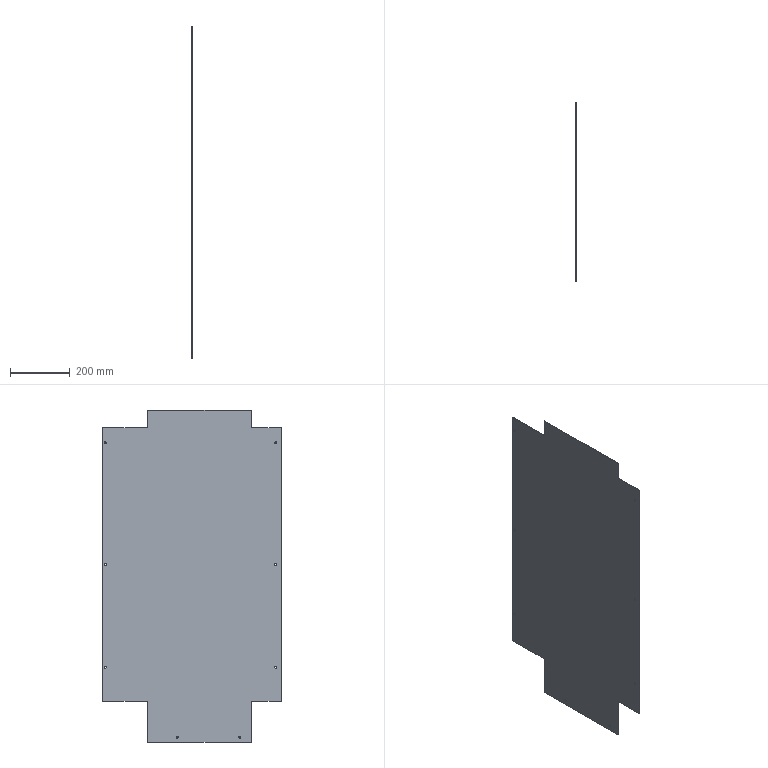Part | NX | 1 solid | 42 faces | box 2 x 600 x 1110 mm | volume 1233118 mm3 | cylinder 24 | plane 14 | cone 4 | commonest cylinder face diameters 7 x16 4 x8
STEP:
#1=CARTESIAN_POINT('',(1.,-205.,-433.5));
#2=VERTEX_POINT('',#1);
#3=CARTESIAN_POINT('',(1.,-303.,-433.5));
#4=VERTEX_POINT('',#3);
#5=CARTESIAN_POINT('',(1.,0.,-433.5));
#6=DIRECTION('',(0.,-1.,0.));
#7=VECTOR('',#6,1000.);
#8=LINE('',#5,#7);
#9=EDGE_CURVE('',#2,#4,#8,.T.);
#10=ORIENTED_EDGE('',*,*,#9,.F.);
#11=CARTESIAN_POINT('',(1.,-205.,-568.));
#12=VERTEX_POINT('',#11);
#13=CARTESIAN_POINT('',(1.,-205.,0.));
#14=DIRECTION('',(0.,0.,-1.));
#15=VECTOR('',#14,1000.);
#16=LINE('',#13,#15);
#17=EDGE_CURVE('',#2,#12,#16,.T.);
#18=ORIENTED_EDGE('',*,*,#17,.T.);
#19=CARTESIAN_POINT('',(1.,-203.,-570.));
#20=VERTEX_POINT('',#19);
#21=CARTESIAN_POINT('',(1.,-203.,-568.));
#22=DIRECTION('',(-1.,0.,0.));
#23=DIRECTION('',(0.,1.,0.));
#24=AXIS2_PLACEMENT_3D('',#21,#22,#23);
#25=CIRCLE('',#24,2.);
#26=EDGE_CURVE('',#20,#12,#25,.T.);
#27=ORIENTED_EDGE('',*,*,#26,.F.);
#28=CARTESIAN_POINT('',(1.,143.,-570.));
#29=VERTEX_POINT('',#28);
#30=CARTESIAN_POINT('',(1.,0.,-570.));
#31=DIRECTION('',(0.,-1.,0.));
#32=VECTOR('',#31,1000.);
#33=LINE('',#30,#32);
#34=EDGE_CURVE('',#29,#20,#33,.T.);
#35=ORIENTED_EDGE('',*,*,#34,.F.);
#36=CARTESIAN_POINT('',(1.,145.,-568.));
#37=VERTEX_POINT('',#36);
#38=CARTESIAN_POINT('',(1.,143.,-568.));
#39=DIRECTION('',(-1.,0.,0.));
#40=DIRECTION('',(0.,1.,0.));
#41=AXIS2_PLACEMENT_3D('',#38,#39,#40);
#42=CIRCLE('',#41,2.);
#43=EDGE_CURVE('',#37,#29,#42,.T.);
#44=ORIENTED_EDGE('',*,*,#43,.F.);
#45=CARTESIAN_POINT('',(1.,145.,-433.5));
#46=VERTEX_POINT('',#45);
#47=CARTESIAN_POINT('',(1.,145.,0.));
#48=DIRECTION('',(0.,0.,-1.));
#49=VECTOR('',#48,1000.);
#50=LINE('',#47,#49);
#51=EDGE_CURVE('',#46,#37,#50,.T.);
#52=ORIENTED_EDGE('',*,*,#51,.F.);
#53=CARTESIAN_POINT('',(1.,293.,-433.5));
#54=VERTEX_POINT('',#53);
#55=CARTESIAN_POINT('',(1.,0.,-433.5));
#56=DIRECTION('',(0.,-1.,0.));
#57=VECTOR('',#56,1000.);
#58=LINE('',#55,#57);
#59=EDGE_CURVE('',#54,#46,#58,.T.);
#60=ORIENTED_EDGE('',*,*,#59,.F.);
#61=CARTESIAN_POINT('',(1.,295.,-431.5));
#62=VERTEX_POINT('',#61);
#63=CARTESIAN_POINT('',(1.,293.,-431.5));
#64=DIRECTION('',(1.,0.,0.));
#65=DIRECTION('',(0.,-1.,0.));
#66=AXIS2_PLACEMENT_3D('',#63,#64,#65);
#67=CIRCLE('',#66,2.);
#68=EDGE_CURVE('',#54,#62,#67,.T.);
#69=ORIENTED_EDGE('',*,*,#68,.T.);
#70=CARTESIAN_POINT('',(1.,295.,478.));
#71=VERTEX_POINT('',#70);
#72=CARTESIAN_POINT('',(1.,295.,0.));
#73=DIRECTION('',(0.,0.,-1.));
#74=VECTOR('',#73,1000.);
#75=LINE('',#72,#74);
#76=EDGE_CURVE('',#71,#62,#75,.T.);
#77=ORIENTED_EDGE('',*,*,#76,.F.);
#78=CARTESIAN_POINT('',(1.,293.,480.));
#79=VERTEX_POINT('',#78);
#80=CARTESIAN_POINT('',(1.,293.,478.));
#81=DIRECTION('',(-1.,0.,0.));
#82=DIRECTION('',(0.,1.,0.));
#83=AXIS2_PLACEMENT_3D('',#80,#81,#82);
#84=CIRCLE('',#83,2.);
#85=EDGE_CURVE('',#79,#71,#84,.T.);
#86=ORIENTED_EDGE('',*,*,#85,.F.);
#87=CARTESIAN_POINT('',(1.,145.,480.));
#88=VERTEX_POINT('',#87);
#89=CARTESIAN_POINT('',(1.,0.,480.));
#90=DIRECTION('',(0.,-1.,0.));
#91=VECTOR('',#90,1000.);
#92=LINE('',#89,#91);
#93=EDGE_CURVE('',#79,#88,#92,.T.);
#94=ORIENTED_EDGE('',*,*,#93,.T.);
#95=CARTESIAN_POINT('',(1.,145.,538.));
#96=VERTEX_POINT('',#95);
#97=CARTESIAN_POINT('',(1.,145.,0.));
#98=DIRECTION('',(0.,0.,1.));
#99=VECTOR('',#98,1000.);
#100=LINE('',#97,#99);
#101=EDGE_CURVE('',#88,#96,#100,.T.);
#102=ORIENTED_EDGE('',*,*,#101,.T.);
#103=CARTESIAN_POINT('',(1.,143.,540.));
#104=VERTEX_POINT('',#103);
#105=CARTESIAN_POINT('',(1.,143.,538.));
#106=DIRECTION('',(-1.,0.,0.));
#107=DIRECTION('',(0.,1.,0.));
#108=AXIS2_PLACEMENT_3D('',#105,#106,#107);
#109=CIRCLE('',#108,2.);
#110=EDGE_CURVE('',#104,#96,#109,.T.);
#111=ORIENTED_EDGE('',*,*,#110,.F.);
#112=CARTESIAN_POINT('',(1.,-203.,540.));
#113=VERTEX_POINT('',#112);
#114=CARTESIAN_POINT('',(1.,0.,540.));
#115=DIRECTION('',(0.,-1.,0.));
#116=VECTOR('',#115,1000.);
#117=LINE('',#114,#116);
#118=EDGE_CURVE('',#104,#113,#117,.T.);
#119=ORIENTED_EDGE('',*,*,#118,.T.);
#120=CARTESIAN_POINT('',(1.,-205.,538.));
#121=VERTEX_POINT('',#120);
#122=CARTESIAN_POINT('',(1.,-203.,538.));
#123=DIRECTION('',(1.,0.,0.));
#124=DIRECTION('',(0.,-1.,0.));
#125=AXIS2_PLACEMENT_3D('',#122,#123,#124);
#126=CIRCLE('',#125,2.);
#127=EDGE_CURVE('',#113,#121,#126,.T.);
#128=ORIENTED_EDGE('',*,*,#127,.T.);
#129=CARTESIAN_POINT('',(1.,-205.,480.));
#130=VERTEX_POINT('',#129);
#131=CARTESIAN_POINT('',(1.,-205.,0.));
#132=DIRECTION('',(0.,0.,-1.));
#133=VECTOR('',#132,1000.);
#134=LINE('',#131,#133);
#135=EDGE_CURVE('',#121,#130,#134,.T.);
#136=ORIENTED_EDGE('',*,*,#135,.T.);
#137=CARTESIAN_POINT('',(1.,-303.,480.));
#138=VERTEX_POINT('',#137);
#139=CARTESIAN_POINT('',(1.,0.,480.));
#140=DIRECTION('',(0.,-1.,0.));
#141=VECTOR('',#140,1000.);
#142=LINE('',#139,#141);
#143=EDGE_CURVE('',#130,#138,#142,.T.);
#144=ORIENTED_EDGE('',*,*,#143,.T.);
#145=CARTESIAN_POINT('',(1.,-305.,478.));
#146=VERTEX_POINT('',#145);
#147=CARTESIAN_POINT('',(1.,-303.,478.));
#148=DIRECTION('',(-1.,0.,0.));
#149=DIRECTION('',(0.,1.,0.));
#150=AXIS2_PLACEMENT_3D('',#147,#148,#149);
#151=CIRCLE('',#150,2.);
#152=EDGE_CURVE('',#146,#138,#151,.T.);
#153=ORIENTED_EDGE('',*,*,#152,.F.);
#154=CARTESIAN_POINT('',(1.,-305.,-431.5));
#155=VERTEX_POINT('',#154);
#156=CARTESIAN_POINT('',(1.,-305.,0.));
#157=DIRECTION('',(0.,0.,-1.));
#158=VECTOR('',#157,1000.);
#159=LINE('',#156,#158);
#160=EDGE_CURVE('',#146,#155,#159,.T.);
#161=ORIENTED_EDGE('',*,*,#160,.T.);
#162=CARTESIAN_POINT('',(1.,-303.,-431.5));
#163=DIRECTION('',(1.,0.,0.));
#164=DIRECTION('',(0.,-1.,0.));
#165=AXIS2_PLACEMENT_3D('',#162,#163,#164);
#166=CIRCLE('',#165,2.);
#167=EDGE_CURVE('',#155,#4,#166,.T.);
#168=ORIENTED_EDGE('',*,*,#167,.T.);
#169=EDGE_LOOP('',(#10,#18,#27,#35,#44,#52,#60,#69,#77,#86,#94,#102,#111,#119,#128,#136,#144,#153,#161,#168));
#170=FACE_BOUND('',#169,.T.);
#171=CARTESIAN_POINT('',(1.,-165.,-557.));
#172=VERTEX_POINT('',#171);
#173=CARTESIAN_POINT('',(1.,-165.,-550.));
#174=VERTEX_POINT('',#173);
#175=CARTESIAN_POINT('',(1.,-165.,-553.5));
#176=DIRECTION('',(-1.,0.,0.));
#177=DIRECTION('',(0.,0.,1.));
#178=AXIS2_PLACEMENT_3D('',#175,#176,#177);
#179=CIRCLE('',#178,3.5);
#180=EDGE_CURVE('',#172,#174,#179,.T.);
#181=ORIENTED_EDGE('',*,*,#180,.T.);
#182=CARTESIAN_POINT('',(1.,-165.,-553.5));
#183=DIRECTION('',(-1.,0.,0.));
#184=DIRECTION('',(0.,0.,1.));
#185=AXIS2_PLACEMENT_3D('',#182,#183,#184);
#186=CIRCLE('',#185,3.5);
#187=EDGE_CURVE('',#174,#172,#186,.T.);
#188=ORIENTED_EDGE('',*,*,#187,.T.);
#189=EDGE_LOOP('',(#181,#188));
#190=FACE_BOUND('',#189,.T.);
#191=CARTESIAN_POINT('',(1.,-288.5,430.));
#192=VERTEX_POINT('',#191);
#193=CARTESIAN_POINT('',(1.,-281.5,430.));
#194=VERTEX_POINT('',#193);
#195=CARTESIAN_POINT('',(1.,-285.,430.));
#196=DIRECTION('',(1.,0.,0.));
#197=DIRECTION('',(0.,1.,0.));
#198=AXIS2_PLACEMENT_3D('',#195,#196,#197);
#199=CIRCLE('',#198,3.5);
#200=EDGE_CURVE('',#192,#194,#199,.T.);
#201=ORIENTED_EDGE('',*,*,#200,.F.);
#202=CARTESIAN_POINT('',(1.,-285.,430.));
#203=DIRECTION('',(1.,0.,0.));
#204=DIRECTION('',(0.,1.,0.));
#205=AXIS2_PLACEMENT_3D('',#202,#203,#204);
#206=CIRCLE('',#205,3.5);
#207=EDGE_CURVE('',#194,#192,#206,.T.);
#208=ORIENTED_EDGE('',*,*,#207,.F.);
#209=EDGE_LOOP('',(#201,#208));
#210=FACE_BOUND('',#209,.T.);
#211=CARTESIAN_POINT('',(1.,45.,-557.));
#212=VERTEX_POINT('',#211);
#213=CARTESIAN_POINT('',(1.,45.,-550.));
#214=VERTEX_POINT('',#213);
#215=CARTESIAN_POINT('',(1.,45.,-553.5));
#216=DIRECTION('',(-1.,0.,0.));
#217=DIRECTION('',(0.,0.,1.));
#218=AXIS2_PLACEMENT_3D('',#215,#216,#217);
#219=CIRCLE('',#218,3.5);
#220=EDGE_CURVE('',#212,#214,#219,.T.);
#221=ORIENTED_EDGE('',*,*,#220,.T.);
#222=CARTESIAN_POINT('',(1.,45.,-553.5));
#223=DIRECTION('',(-1.,0.,0.));
#224=DIRECTION('',(0.,0.,1.));
#225=AXIS2_PLACEMENT_3D('',#222,#223,#224);
#226=CIRCLE('',#225,3.5);
#227=EDGE_CURVE('',#214,#212,#226,.T.);
#228=ORIENTED_EDGE('',*,*,#227,.T.);
#229=EDGE_LOOP('',(#221,#228));
#230=FACE_BOUND('',#229,.T.);
#231=CARTESIAN_POINT('',(1.,-281.2,23.25));
#232=VERTEX_POINT('',#231);
#233=CARTESIAN_POINT('',(1.,-288.8,23.25));
#234=VERTEX_POINT('',#233);
#235=CARTESIAN_POINT('',(1.,-285.,23.25));
#236=DIRECTION('',(1.,0.,0.));
#237=DIRECTION('',(0.,-1.,0.));
#238=AXIS2_PLACEMENT_3D('',#235,#236,#237);
#239=CIRCLE('',#238,3.8);
#240=EDGE_CURVE('',#232,#234,#239,.T.);
#241=ORIENTED_EDGE('',*,*,#240,.F.);
#242=CARTESIAN_POINT('',(1.,-285.,23.25));
#243=DIRECTION('',(1.,0.,0.));
#244=DIRECTION('',(0.,-1.,0.));
#245=AXIS2_PLACEMENT_3D('',#242,#243,#244);
#246=CIRCLE('',#245,3.8);
#247=EDGE_CURVE('',#234,#232,#246,.T.);
#248=ORIENTED_EDGE('',*,*,#247,.F.);
#249=EDGE_LOOP('',(#241,#248));
#250=FACE_BOUND('',#249,.T.);
#251=CARTESIAN_POINT('',(1.,-288.5,-320.));
#252=VERTEX_POINT('',#251);
#253=CARTESIAN_POINT('',(1.,-281.5,-320.));
#254=VERTEX_POINT('',#253);
#255=CARTESIAN_POINT('',(1.,-285.,-320.));
#256=DIRECTION('',(1.,0.,0.));
#257=DIRECTION('',(0.,1.,0.));
#258=AXIS2_PLACEMENT_3D('',#255,#256,#257);
#259=CIRCLE('',#258,3.5);
#260=EDGE_CURVE('',#252,#254,#259,.T.);
#261=ORIENTED_EDGE('',*,*,#260,.F.);
#262=CARTESIAN_POINT('',(1.,-285.,-320.));
#263=DIRECTION('',(1.,0.,0.));
#264=DIRECTION('',(0.,1.,0.));
#265=AXIS2_PLACEMENT_3D('',#262,#263,#264);
#266=CIRCLE('',#265,3.5);
#267=EDGE_CURVE('',#254,#252,#266,.T.);
#268=ORIENTED_EDGE('',*,*,#267,.F.);
#269=EDGE_LOOP('',(#261,#268));
#270=FACE_BOUND('',#269,.T.);
#271=CARTESIAN_POINT('',(1.,281.5,430.));
#272=VERTEX_POINT('',#271);
#273=CARTESIAN_POINT('',(1.,288.5,430.));
#274=VERTEX_POINT('',#273);
#275=CARTESIAN_POINT('',(1.,285.,430.));
#276=DIRECTION('',(1.,0.,0.));
#277=DIRECTION('',(0.,1.,0.));
#278=AXIS2_PLACEMENT_3D('',#275,#276,#277);
#279=CIRCLE('',#278,3.5);
#280=EDGE_CURVE('',#272,#274,#279,.T.);
#281=ORIENTED_EDGE('',*,*,#280,.F.);
#282=CARTESIAN_POINT('',(1.,285.,430.));
#283=DIRECTION('',(1.,0.,0.));
#284=DIRECTION('',(0.,1.,0.));
#285=AXIS2_PLACEMENT_3D('',#282,#283,#284);
#286=CIRCLE('',#285,3.5);
#287=EDGE_CURVE('',#274,#272,#286,.T.);
#288=ORIENTED_EDGE('',*,*,#287,.F.);
#289=EDGE_LOOP('',(#281,#288));
#290=FACE_BOUND('',#289,.T.);
#291=CARTESIAN_POINT('',(1.,288.8,23.25));
#292=VERTEX_POINT('',#291);
#293=CARTESIAN_POINT('',(1.,281.2,23.25));
#294=VERTEX_POINT('',#293);
#295=CARTESIAN_POINT('',(1.,285.,23.25));
#296=DIRECTION('',(1.,0.,0.));
#297=DIRECTION('',(0.,-1.,0.));
#298=AXIS2_PLACEMENT_3D('',#295,#296,#297);
#299=CIRCLE('',#298,3.8);
#300=EDGE_CURVE('',#292,#294,#299,.T.);
#301=ORIENTED_EDGE('',*,*,#300,.F.);
#302=CARTESIAN_POINT('',(1.,285.,23.25));
#303=DIRECTION('',(1.,0.,0.));
#304=DIRECTION('',(0.,-1.,0.));
#305=AXIS2_PLACEMENT_3D('',#302,#303,#304);
#306=CIRCLE('',#305,3.8);
#307=EDGE_CURVE('',#294,#292,#306,.T.);
#308=ORIENTED_EDGE('',*,*,#307,.F.);
#309=EDGE_LOOP('',(#301,#308));
#310=FACE_BOUND('',#309,.T.);
#311=CARTESIAN_POINT('',(1.,281.5,-320.));
#312=VERTEX_POINT('',#311);
#313=CARTESIAN_POINT('',(1.,288.5,-320.));
#314=VERTEX_POINT('',#313);
#315=CARTESIAN_POINT('',(1.,285.,-320.));
#316=DIRECTION('',(1.,0.,0.));
#317=DIRECTION('',(0.,1.,0.));
#318=AXIS2_PLACEMENT_3D('',#315,#316,#317);
#319=CIRCLE('',#318,3.5);
#320=EDGE_CURVE('',#312,#314,#319,.T.);
#321=ORIENTED_EDGE('',*,*,#320,.F.);
#322=CARTESIAN_POINT('',(1.,285.,-320.));
#323=DIRECTION('',(1.,0.,0.));
#324=DIRECTION('',(0.,1.,0.));
#325=AXIS2_PLACEMENT_3D('',#322,#323,#324);
#326=CIRCLE('',#325,3.5);
#327=EDGE_CURVE('',#314,#312,#326,.T.);
#328=ORIENTED_EDGE('',*,*,#327,.F.);
#329=EDGE_LOOP('',(#321,#328));
#330=FACE_BOUND('',#329,.T.);
#331=CARTESIAN_POINT('',(1.,0.,0.));
#332=DIRECTION('',(1.,0.,0.));
#333=DIRECTION('',(0.,1.,0.));
#334=AXIS2_PLACEMENT_3D('',#331,#332,#333);
#335=PLANE('',#334);
#336=ADVANCED_FACE('',(#170,#190,#210,#230,#250,#270,#290,#310,#330),#335,.T.);
#337=CARTESIAN_POINT('',(-1.,-303.,-433.5));
#338=VERTEX_POINT('',#337);
#339=CARTESIAN_POINT('',(0.,-303.,-433.5));
#340=DIRECTION('',(1.,0.,0.));
#341=VECTOR('',#340,1000.);
#342=LINE('',#339,#341);
#343=EDGE_CURVE('',#338,#4,#342,.T.);
#344=ORIENTED_EDGE('',*,*,#343,.F.);
#345=CARTESIAN_POINT('',(-1.,-205.,-433.5));
#346=VERTEX_POINT('',#345);
#347=CARTESIAN_POINT('',(-1.,0.,-433.5));
#348=DIRECTION('',(0.,-1.,0.));
#349=VECTOR('',#348,1000.);
#350=LINE('',#347,#349);
#351=EDGE_CURVE('',#346,#338,#350,.T.);
#352=ORIENTED_EDGE('',*,*,#351,.F.);
#353=CARTESIAN_POINT('',(0.,-205.,-433.5));
#354=DIRECTION('',(1.,0.,0.));
#355=VECTOR('',#354,1000.);
#356=LINE('',#353,#355);
#357=EDGE_CURVE('',#346,#2,#356,.T.);
#358=ORIENTED_EDGE('',*,*,#357,.T.);
#359=ORIENTED_EDGE('',*,*,#9,.T.);
#360=EDGE_LOOP('',(#344,#352,#358,#359));
#361=FACE_BOUND('',#360,.T.);
#362=CARTESIAN_POINT('',(-1.,-295.,-433.5));
#363=DIRECTION('',(0.,0.,1.));
#364=DIRECTION('',(1.,0.,0.));
#365=AXIS2_PLACEMENT_3D('',#362,#363,#364);
#366=PLANE('',#365);
#367=ADVANCED_FACE('',(#361),#366,.F.);
#368=CARTESIAN_POINT('',(-1.,-305.,478.));
#369=VERTEX_POINT('',#368);
#370=CARTESIAN_POINT('',(0.,-305.,478.));
#371=DIRECTION('',(-1.,0.,0.));
#372=VECTOR('',#371,1000.);
#373=LINE('',#370,#372);
#374=EDGE_CURVE('',#146,#369,#373,.T.);
#375=ORIENTED_EDGE('',*,*,#374,.T.);
#376=CARTESIAN_POINT('',(-1.,-305.,-431.5));
#377=VERTEX_POINT('',#376);
#378=CARTESIAN_POINT('',(-1.,-305.,0.));
#379=DIRECTION('',(0.,0.,-1.));
#380=VECTOR('',#379,1000.);
#381=LINE('',#378,#380);
#382=EDGE_CURVE('',#369,#377,#381,.T.);
#383=ORIENTED_EDGE('',*,*,#382,.T.);
#384=CARTESIAN_POINT('',(0.,-305.,-431.5));
#385=DIRECTION('',(1.,0.,0.));
#386=VECTOR('',#385,1000.);
#387=LINE('',#384,#386);
#388=EDGE_CURVE('',#377,#155,#387,.T.);
#389=ORIENTED_EDGE('',*,*,#388,.T.);
#390=ORIENTED_EDGE('',*,*,#160,.F.);
#391=EDGE_LOOP('',(#375,#383,#389,#390));
#392=FACE_BOUND('',#391,.T.);
#393=CARTESIAN_POINT('',(-1.,-305.,570.));
#394=DIRECTION('',(0.,-1.,0.));
#395=DIRECTION('',(0.,0.,-1.));
#396=AXIS2_PLACEMENT_3D('',#393,#394,#395);
#397=PLANE('',#396);
#398=ADVANCED_FACE('',(#392),#397,.T.);
#399=CARTESIAN_POINT('',(-1.,-205.,480.));
#400=VERTEX_POINT('',#399);
#401=CARTESIAN_POINT('',(-1.,-303.,480.));
#402=VERTEX_POINT('',#401);
#403=CARTESIAN_POINT('',(-1.,0.,480.));
#404=DIRECTION('',(0.,-1.,0.));
#405=VECTOR('',#404,1000.);
#406=LINE('',#403,#405);
#407=EDGE_CURVE('',#400,#402,#406,.T.);
#408=ORIENTED_EDGE('',*,*,#407,.T.);
#409=CARTESIAN_POINT('',(0.,-303.,480.));
#410=DIRECTION('',(-1.,0.,0.));
#411=VECTOR('',#410,1000.);
#412=LINE('',#409,#411);
#413=EDGE_CURVE('',#138,#402,#412,.T.);
#414=ORIENTED_EDGE('',*,*,#413,.F.);
#415=ORIENTED_EDGE('',*,*,#143,.F.);
#416=CARTESIAN_POINT('',(1.,-205.,480.));
#417=DIRECTION('',(-1.,0.,0.));
#418=VECTOR('',#417,1000.);
#419=LINE('',#416,#418);
#420=EDGE_CURVE('',#130,#400,#419,.T.);
#421=ORIENTED_EDGE('',*,*,#420,.T.);
#422=EDGE_LOOP('',(#408,#414,#415,#421));
#423=FACE_BOUND('',#422,.T.);
#424=CARTESIAN_POINT('',(-1.,-205.,480.));
#425=DIRECTION('',(0.,0.,-1.));
#426=DIRECTION('',(0.,-1.,0.));
#427=AXIS2_PLACEMENT_3D('',#424,#425,#426);
#428=PLANE('',#427);
#429=ADVANCED_FACE('',(#423),#428,.F.);
#430=CARTESIAN_POINT('',(-1.,-205.,538.));
#431=VERTEX_POINT('',#430);
#432=CARTESIAN_POINT('',(0.,-205.,538.));
#433=DIRECTION('',(1.,0.,0.));
#434=VECTOR('',#433,1000.);
#435=LINE('',#432,#434);
#436=EDGE_CURVE('',#431,#121,#435,.T.);
#437=ORIENTED_EDGE('',*,*,#436,.F.);
#438=CARTESIAN_POINT('',(-1.,-205.,0.));
#439=DIRECTION('',(0.,0.,-1.));
#440=VECTOR('',#439,1000.);
#441=LINE('',#438,#440);
#442=EDGE_CURVE('',#431,#400,#441,.T.);
#443=ORIENTED_EDGE('',*,*,#442,.T.);
#444=ORIENTED_EDGE('',*,*,#420,.F.);
#445=ORIENTED_EDGE('',*,*,#135,.F.);
#446=EDGE_LOOP('',(#437,#443,#444,#445));
#447=FACE_BOUND('',#446,.T.);
#448=CARTESIAN_POINT('',(-1.,-205.,570.));
#449=DIRECTION('',(0.,1.,0.));
#450=DIRECTION('',(1.,0.,0.));
#451=AXIS2_PLACEMENT_3D('',#448,#449,#450);
#452=PLANE('',#451);
#453=ADVANCED_FACE('',(#447),#452,.F.);
#454=CARTESIAN_POINT('',(-1.,143.,540.));
#455=VERTEX_POINT('',#454);
#456=CARTESIAN_POINT('',(0.,143.,540.));
#457=DIRECTION('',(-1.,0.,0.));
#458=VECTOR('',#457,1000.);
#459=LINE('',#456,#458);
#460=EDGE_CURVE('',#104,#455,#459,.T.);
#461=ORIENTED_EDGE('',*,*,#460,.T.);
#462=CARTESIAN_POINT('',(-1.,-203.,540.));
#463=VERTEX_POINT('',#462);
#464=CARTESIAN_POINT('',(-1.,0.,540.));
#465=DIRECTION('',(0.,-1.,0.));
#466=VECTOR('',#465,1000.);
#467=LINE('',#464,#466);
#468=EDGE_CURVE('',#455,#463,#467,.T.);
#469=ORIENTED_EDGE('',*,*,#468,.T.);
#470=CARTESIAN_POINT('',(0.,-203.,540.));
#471=DIRECTION('',(1.,0.,0.));
#472=VECTOR('',#471,1000.);
#473=LINE('',#470,#472);
#474=EDGE_CURVE('',#463,#113,#473,.T.);
#475=ORIENTED_EDGE('',*,*,#474,.T.);
#476=ORIENTED_EDGE('',*,*,#118,.F.);
#477=EDGE_LOOP('',(#461,#469,#475,#476));
#478=FACE_BOUND('',#477,.T.);
#479=CARTESIAN_POINT('',(-1.,295.,540.));
#480=DIRECTION('',(0.,0.,1.));
#481=DIRECTION('',(1.,0.,0.));
#482=AXIS2_PLACEMENT_3D('',#479,#480,#481);
#483=PLANE('',#482);
#484=ADVANCED_FACE('',(#478),#483,.T.);
#485=CARTESIAN_POINT('',(-1.,145.,480.));
#486=VERTEX_POINT('',#485);
#487=CARTESIAN_POINT('',(-1.,145.,538.));
#488=VERTEX_POINT('',#487);
#489=CARTESIAN_POINT('',(-1.,145.,0.));
#490=DIRECTION('',(0.,0.,1.));
#491=VECTOR('',#490,1000.);
#492=LINE('',#489,#491);
#493=EDGE_CURVE('',#486,#488,#492,.T.);
#494=ORIENTED_EDGE('',*,*,#493,.T.);
#495=CARTESIAN_POINT('',(0.,145.,538.));
#496=DIRECTION('',(-1.,0.,0.));
#497=VECTOR('',#496,1000.);
#498=LINE('',#495,#497);
#499=EDGE_CURVE('',#96,#488,#498,.T.);
#500=ORIENTED_EDGE('',*,*,#499,.F.);
#501=ORIENTED_EDGE('',*,*,#101,.F.);
#502=CARTESIAN_POINT('',(1.,145.,480.));
#503=DIRECTION('',(-1.,0.,0.));
#504=VECTOR('',#503,1000.);
#505=LINE('',#502,#504);
#506=EDGE_CURVE('',#88,#486,#505,.T.);
#507=ORIENTED_EDGE('',*,*,#506,.T.);
#508=EDGE_LOOP('',(#494,#500,#501,#507));
#509=FACE_BOUND('',#508,.T.);
#510=CARTESIAN_POINT('',(-1.,145.,480.));
#511=DIRECTION('',(0.,-1.,0.));
#512=DIRECTION('',(0.,0.,-1.));
#513=AXIS2_PLACEMENT_3D('',#510,#511,#512);
#514=PLANE('',#513);
#515=ADVANCED_FACE('',(#509),#514,.F.);
#516=CARTESIAN_POINT('',(-1.,293.,480.));
#517=VERTEX_POINT('',#516);
#518=CARTESIAN_POINT('',(0.,293.,480.));
#519=DIRECTION('',(-1.,0.,0.));
#520=VECTOR('',#519,1000.);
#521=LINE('',#518,#520);
#522=EDGE_CURVE('',#79,#517,#521,.T.);
#523=ORIENTED_EDGE('',*,*,#522,.T.);
#524=CARTESIAN_POINT('',(-1.,0.,480.));
#525=DIRECTION('',(0.,-1.,0.));
#526=VECTOR('',#525,1000.);
#527=LINE('',#524,#526);
#528=EDGE_CURVE('',#517,#486,#527,.T.);
#529=ORIENTED_EDGE('',*,*,#528,.T.);
#530=ORIENTED_EDGE('',*,*,#506,.F.);
#531=ORIENTED_EDGE('',*,*,#93,.F.);
#532=EDGE_LOOP('',(#523,#529,#530,#531));
#533=FACE_BOUND('',#532,.T.);
#534=CARTESIAN_POINT('',(-1.,295.,480.));
#535=DIRECTION('',(0.,0.,-1.));
#536=DIRECTION('',(0.,-1.,0.));
#537=AXIS2_PLACEMENT_3D('',#534,#535,#536);
#538=PLANE('',#537);
#539=ADVANCED_FACE('',(#533),#538,.F.);
#540=CARTESIAN_POINT('',(-1.,295.,-431.5));
#541=VERTEX_POINT('',#540);
#542=CARTESIAN_POINT('',(0.,295.,-431.5));
#543=DIRECTION('',(1.,0.,0.));
#544=VECTOR('',#543,1000.);
#545=LINE('',#542,#544);
#546=EDGE_CURVE('',#541,#62,#545,.T.);
#547=ORIENTED_EDGE('',*,*,#546,.F.);
#548=CARTESIAN_POINT('',(-1.,295.,478.));
#549=VERTEX_POINT('',#548);
#550=CARTESIAN_POINT('',(-1.,295.,0.));
#551=DIRECTION('',(0.,0.,-1.));
#552=VECTOR('',#551,1000.);
#553=LINE('',#550,#552);
#554=EDGE_CURVE('',#549,#541,#553,.T.);
#555=ORIENTED_EDGE('',*,*,#554,.F.);
#556=CARTESIAN_POINT('',(0.,295.,478.));
#557=DIRECTION('',(-1.,0.,0.));
#558=VECTOR('',#557,1000.);
#559=LINE('',#556,#558);
#560=EDGE_CURVE('',#71,#549,#559,.T.);
#561=ORIENTED_EDGE('',*,*,#560,.F.);
#562=ORIENTED_EDGE('',*,*,#76,.T.);
#563=EDGE_LOOP('',(#547,#555,#561,#562));
#564=FACE_BOUND('',#563,.T.);
#565=CARTESIAN_POINT('',(-1.,295.,-570.));
#566=DIRECTION('',(0.,1.,0.));
#567=DIRECTION('',(1.,0.,0.));
#568=AXIS2_PLACEMENT_3D('',#565,#566,#567);
#569=PLANE('',#568);
#570=ADVANCED_FACE('',(#564),#569,.T.);
#571=CARTESIAN_POINT('',(-1.,293.,-433.5));
#572=VERTEX_POINT('',#571);
#573=CARTESIAN_POINT('',(-1.,145.,-433.5));
#574=VERTEX_POINT('',#573);
#575=CARTESIAN_POINT('',(-1.,0.,-433.5));
#576=DIRECTION('',(0.,-1.,0.));
#577=VECTOR('',#576,1000.);
#578=LINE('',#575,#577);
#579=EDGE_CURVE('',#572,#574,#578,.T.);
#580=ORIENTED_EDGE('',*,*,#579,.F.);
#581=CARTESIAN_POINT('',(0.,293.,-433.5));
#582=DIRECTION('',(1.,0.,0.));
#583=VECTOR('',#582,1000.);
#584=LINE('',#581,#583);
#585=EDGE_CURVE('',#572,#54,#584,.T.);
#586=ORIENTED_EDGE('',*,*,#585,.T.);
#587=ORIENTED_EDGE('',*,*,#59,.T.);
#588=CARTESIAN_POINT('',(0.,145.,-433.5));
#589=DIRECTION('',(-1.,0.,0.));
#590=VECTOR('',#589,1000.);
#591=LINE('',#588,#590);
#592=EDGE_CURVE('',#46,#574,#591,.T.);
#593=ORIENTED_EDGE('',*,*,#592,.T.);
#594=EDGE_LOOP('',(#580,#586,#587,#593));
#595=FACE_BOUND('',#594,.T.);
#596=CARTESIAN_POINT('',(-1.,105.,-433.5));
#597=DIRECTION('',(0.,0.,1.));
#598=DIRECTION('',(1.,0.,0.));
#599=AXIS2_PLACEMENT_3D('',#596,#597,#598);
#600=PLANE('',#599);
#601=ADVANCED_FACE('',(#595),#600,.F.);
#602=CARTESIAN_POINT('',(-1.,145.,-568.));
#603=VERTEX_POINT('',#602);
#604=CARTESIAN_POINT('',(0.,145.,-568.));
#605=DIRECTION('',(-1.,0.,0.));
#606=VECTOR('',#605,1000.);
#607=LINE('',#604,#606);
#608=EDGE_CURVE('',#37,#603,#607,.T.);
#609=ORIENTED_EDGE('',*,*,#608,.T.);
#610=CARTESIAN_POINT('',(-1.,145.,0.));
#611=DIRECTION('',(0.,0.,-1.));
#612=VECTOR('',#611,1000.);
#613=LINE('',#610,#612);
#614=EDGE_CURVE('',#574,#603,#613,.T.);
#615=ORIENTED_EDGE('',*,*,#614,.F.);
#616=ORIENTED_EDGE('',*,*,#592,.F.);
#617=ORIENTED_EDGE('',*,*,#51,.T.);
#618=EDGE_LOOP('',(#609,#615,#616,#617));
#619=FACE_BOUND('',#618,.T.);
#620=CARTESIAN_POINT('',(-1.,145.,-570.));
#621=DIRECTION('',(0.,-1.,0.));
#622=DIRECTION('',(0.,0.,-1.));
#623=AXIS2_PLACEMENT_3D('',#620,#621,#622);
#624=PLANE('',#623);
#625=ADVANCED_FACE('',(#619),#624,.F.);
#626=CARTESIAN_POINT('',(-1.,-203.,-570.));
#627=VERTEX_POINT('',#626);
#628=CARTESIAN_POINT('',(0.,-203.,-570.));
#629=DIRECTION('',(-1.,0.,0.));
#630=VECTOR('',#629,1000.);
#631=LINE('',#628,#630);
#632=EDGE_CURVE('',#20,#627,#631,.T.);
#633=ORIENTED_EDGE('',*,*,#632,.T.);
#634=CARTESIAN_POINT('',(-1.,143.,-570.));
#635=VERTEX_POINT('',#634);
#636=CARTESIAN_POINT('',(-1.,0.,-570.));
#637=DIRECTION('',(0.,-1.,0.));
#638=VECTOR('',#637,1000.);
#639=LINE('',#636,#638);
#640=EDGE_CURVE('',#635,#627,#639,.T.);
#641=ORIENTED_EDGE('',*,*,#640,.F.);
#642=CARTESIAN_POINT('',(0.,143.,-570.));
#643=DIRECTION('',(-1.,0.,0.));
#644=VECTOR('',#643,1000.);
#645=LINE('',#642,#644);
#646=EDGE_CURVE('',#29,#635,#645,.T.);
#647=ORIENTED_EDGE('',*,*,#646,.F.);
#648=ORIENTED_EDGE('',*,*,#34,.T.);
#649=EDGE_LOOP('',(#633,#641,#647,#648));
#650=FACE_BOUND('',#649,.T.);
#651=CARTESIAN_POINT('',(-1.,-295.,-570.));
#652=DIRECTION('',(0.,0.,-1.));
#653=DIRECTION('',(0.,-1.,0.));
#654=AXIS2_PLACEMENT_3D('',#651,#652,#653);
#655=PLANE('',#654);
#656=ADVANCED_FACE('',(#650),#655,.T.);
#657=CARTESIAN_POINT('',(-1.,-205.,-568.));
#658=VERTEX_POINT('',#657);
#659=CARTESIAN_POINT('',(-1.,-205.,0.));
#660=DIRECTION('',(0.,0.,-1.));
#661=VECTOR('',#660,1000.);
#662=LINE('',#659,#661);
#663=EDGE_CURVE('',#346,#658,#662,.T.);
#664=ORIENTED_EDGE('',*,*,#663,.T.);
#665=CARTESIAN_POINT('',(0.,-205.,-568.));
#666=DIRECTION('',(-1.,0.,0.));
#667=VECTOR('',#666,1000.);
#668=LINE('',#665,#667);
#669=EDGE_CURVE('',#12,#658,#668,.T.);
#670=ORIENTED_EDGE('',*,*,#669,.F.);
#671=ORIENTED_EDGE('',*,*,#17,.F.);
#672=ORIENTED_EDGE('',*,*,#357,.F.);
#673=EDGE_LOOP('',(#664,#670,#671,#672));
#674=FACE_BOUND('',#673,.T.);
#675=CARTESIAN_POINT('',(-1.,-205.,-520.));
#676=DIRECTION('',(0.,1.,0.));
#677=DIRECTION('',(1.,0.,0.));
#678=AXIS2_PLACEMENT_3D('',#675,#676,#677);
#679=PLANE('',#678);
#680=ADVANCED_FACE('',(#674),#679,.F.);
#681=ORIENTED_EDGE('',*,*,#351,.T.);
#682=CARTESIAN_POINT('',(-1.,-303.,-431.5));
#683=DIRECTION('',(1.,0.,0.));
#684=DIRECTION('',(0.,-1.,0.));
#685=AXIS2_PLACEMENT_3D('',#682,#683,#684);
#686=CIRCLE('',#685,2.);
#687=EDGE_CURVE('',#377,#338,#686,.T.);
#688=ORIENTED_EDGE('',*,*,#687,.F.);
#689=ORIENTED_EDGE('',*,*,#382,.F.);
#690=CARTESIAN_POINT('',(-1.,-303.,478.));
#691=DIRECTION('',(-1.,0.,0.));
#692=DIRECTION('',(0.,1.,0.));
#693=AXIS2_PLACEMENT_3D('',#690,#691,#692);
#694=CIRCLE('',#693,2.);
#695=EDGE_CURVE('',#369,#402,#694,.T.);
#696=ORIENTED_EDGE('',*,*,#695,.T.);
#697=ORIENTED_EDGE('',*,*,#407,.F.);
#698=ORIENTED_EDGE('',*,*,#442,.F.);
#699=CARTESIAN_POINT('',(-1.,-203.,538.));
#700=DIRECTION('',(1.,0.,0.));
#701=DIRECTION('',(0.,-1.,0.));
#702=AXIS2_PLACEMENT_3D('',#699,#700,#701);
#703=CIRCLE('',#702,2.);
#704=EDGE_CURVE('',#463,#431,#703,.T.);
#705=ORIENTED_EDGE('',*,*,#704,.F.);
#706=ORIENTED_EDGE('',*,*,#468,.F.);
#707=CARTESIAN_POINT('',(-1.,143.,538.));
#708=DIRECTION('',(-1.,0.,0.));
#709=DIRECTION('',(0.,1.,0.));
#710=AXIS2_PLACEMENT_3D('',#707,#708,#709);
#711=CIRCLE('',#710,2.);
#712=EDGE_CURVE('',#455,#488,#711,.T.);
#713=ORIENTED_EDGE('',*,*,#712,.T.);
#714=ORIENTED_EDGE('',*,*,#493,.F.);
#715=ORIENTED_EDGE('',*,*,#528,.F.);
#716=CARTESIAN_POINT('',(-1.,293.,478.));
#717=DIRECTION('',(-1.,0.,0.));
#718=DIRECTION('',(0.,1.,0.));
#719=AXIS2_PLACEMENT_3D('',#716,#717,#718);
#720=CIRCLE('',#719,2.);
#721=EDGE_CURVE('',#517,#549,#720,.T.);
#722=ORIENTED_EDGE('',*,*,#721,.T.);
#723=ORIENTED_EDGE('',*,*,#554,.T.);
#724=CARTESIAN_POINT('',(-1.,293.,-431.5));
#725=DIRECTION('',(1.,0.,0.));
#726=DIRECTION('',(0.,-1.,0.));
#727=AXIS2_PLACEMENT_3D('',#724,#725,#726);
#728=CIRCLE('',#727,2.);
#729=EDGE_CURVE('',#572,#541,#728,.T.);
#730=ORIENTED_EDGE('',*,*,#729,.F.);
#731=ORIENTED_EDGE('',*,*,#579,.T.);
#732=ORIENTED_EDGE('',*,*,#614,.T.);
#733=CARTESIAN_POINT('',(-1.,143.,-568.));
#734=DIRECTION('',(-1.,0.,0.));
#735=DIRECTION('',(0.,1.,0.));
#736=AXIS2_PLACEMENT_3D('',#733,#734,#735);
#737=CIRCLE('',#736,2.);
#738=EDGE_CURVE('',#603,#635,#737,.T.);
#739=ORIENTED_EDGE('',*,*,#738,.T.);
#740=ORIENTED_EDGE('',*,*,#640,.T.);
#741=CARTESIAN_POINT('',(-1.,-203.,-568.));
#742=DIRECTION('',(-1.,0.,0.));
#743=DIRECTION('',(0.,1.,0.));
#744=AXIS2_PLACEMENT_3D('',#741,#742,#743);
#745=CIRCLE('',#744,2.);
#746=EDGE_CURVE('',#627,#658,#745,.T.);
#747=ORIENTED_EDGE('',*,*,#746,.T.);
#748=ORIENTED_EDGE('',*,*,#663,.F.);
#749=EDGE_LOOP('',(#681,#688,#689,#696,#697,#698,#705,#706,#713,#714,#715,#722,#723,#730,#731,#732,#739,#740,#747,#748));
#750=FACE_BOUND('',#749,.T.);
#751=CARTESIAN_POINT('',(-1.,281.5,430.));
#752=VERTEX_POINT('',#751);
#753=CARTESIAN_POINT('',(-1.,288.5,430.));
#754=VERTEX_POINT('',#753);
#755=CARTESIAN_POINT('',(-1.,285.,430.));
#756=DIRECTION('',(1.,0.,0.));
#757=DIRECTION('',(0.,1.,0.));
#758=AXIS2_PLACEMENT_3D('',#755,#756,#757);
#759=CIRCLE('',#758,3.5);
#760=EDGE_CURVE('',#752,#754,#759,.T.);
#761=ORIENTED_EDGE('',*,*,#760,.T.);
#762=CARTESIAN_POINT('',(-1.,285.,430.));
#763=DIRECTION('',(1.,0.,0.));
#764=DIRECTION('',(0.,1.,0.));
#765=AXIS2_PLACEMENT_3D('',#762,#763,#764);
#766=CIRCLE('',#765,3.5);
#767=EDGE_CURVE('',#754,#752,#766,.T.);
#768=ORIENTED_EDGE('',*,*,#767,.T.);
#769=EDGE_LOOP('',(#761,#768));
#770=FACE_BOUND('',#769,.T.);
#771=CARTESIAN_POINT('',(-1.,281.5,-320.));
#772=VERTEX_POINT('',#771);
#773=CARTESIAN_POINT('',(-1.,288.5,-320.));
#774=VERTEX_POINT('',#773);
#775=CARTESIAN_POINT('',(-1.,285.,-320.));
#776=DIRECTION('',(1.,0.,0.));
#777=DIRECTION('',(0.,1.,0.));
#778=AXIS2_PLACEMENT_3D('',#775,#776,#777);
#779=CIRCLE('',#778,3.5);
#780=EDGE_CURVE('',#772,#774,#779,.T.);
#781=ORIENTED_EDGE('',*,*,#780,.T.);
#782=CARTESIAN_POINT('',(-1.,285.,-320.));
#783=DIRECTION('',(1.,0.,0.));
#784=DIRECTION('',(0.,1.,0.));
#785=AXIS2_PLACEMENT_3D('',#782,#783,#784);
#786=CIRCLE('',#785,3.5);
#787=EDGE_CURVE('',#774,#772,#786,.T.);
#788=ORIENTED_EDGE('',*,*,#787,.T.);
#789=EDGE_LOOP('',(#781,#788));
#790=FACE_BOUND('',#789,.T.);
#791=CARTESIAN_POINT('',(-1.,-165.,-557.));
#792=VERTEX_POINT('',#791);
#793=CARTESIAN_POINT('',(-1.,-165.,-550.));
#794=VERTEX_POINT('',#793);
#795=CARTESIAN_POINT('',(-1.,-165.,-553.5));
#796=DIRECTION('',(-1.,0.,0.));
#797=DIRECTION('',(0.,0.,1.));
#798=AXIS2_PLACEMENT_3D('',#795,#796,#797);
#799=CIRCLE('',#798,3.5);
#800=EDGE_CURVE('',#792,#794,#799,.T.);
#801=ORIENTED_EDGE('',*,*,#800,.F.);
#802=CARTESIAN_POINT('',(-1.,-165.,-553.5));
#803=DIRECTION('',(-1.,0.,0.));
#804=DIRECTION('',(0.,0.,1.));
#805=AXIS2_PLACEMENT_3D('',#802,#803,#804);
#806=CIRCLE('',#805,3.5);
#807=EDGE_CURVE('',#794,#792,#806,.T.);
#808=ORIENTED_EDGE('',*,*,#807,.F.);
#809=EDGE_LOOP('',(#801,#808));
#810=FACE_BOUND('',#809,.T.);
#811=CARTESIAN_POINT('',(-1.,-288.5,430.));
#812=VERTEX_POINT('',#811);
#813=CARTESIAN_POINT('',(-1.,-281.5,430.));
#814=VERTEX_POINT('',#813);
#815=CARTESIAN_POINT('',(-1.,-285.,430.));
#816=DIRECTION('',(1.,0.,0.));
#817=DIRECTION('',(0.,1.,0.));
#818=AXIS2_PLACEMENT_3D('',#815,#816,#817);
#819=CIRCLE('',#818,3.5);
#820=EDGE_CURVE('',#812,#814,#819,.T.);
#821=ORIENTED_EDGE('',*,*,#820,.T.);
#822=CARTESIAN_POINT('',(-1.,-285.,430.));
#823=DIRECTION('',(1.,0.,0.));
#824=DIRECTION('',(0.,1.,0.));
#825=AXIS2_PLACEMENT_3D('',#822,#823,#824);
#826=CIRCLE('',#825,3.5);
#827=EDGE_CURVE('',#814,#812,#826,.T.);
#828=ORIENTED_EDGE('',*,*,#827,.T.);
#829=EDGE_LOOP('',(#821,#828));
#830=FACE_BOUND('',#829,.T.);
#831=CARTESIAN_POINT('',(-1.,45.,-557.));
#832=VERTEX_POINT('',#831);
#833=CARTESIAN_POINT('',(-1.,45.,-550.));
#834=VERTEX_POINT('',#833);
#835=CARTESIAN_POINT('',(-1.,45.,-553.5));
#836=DIRECTION('',(-1.,0.,0.));
#837=DIRECTION('',(0.,0.,1.));
#838=AXIS2_PLACEMENT_3D('',#835,#836,#837);
#839=CIRCLE('',#838,3.5);
#840=EDGE_CURVE('',#832,#834,#839,.T.);
#841=ORIENTED_EDGE('',*,*,#840,.F.);
#842=CARTESIAN_POINT('',(-1.,45.,-553.5));
#843=DIRECTION('',(-1.,0.,0.));
#844=DIRECTION('',(0.,0.,1.));
#845=AXIS2_PLACEMENT_3D('',#842,#843,#844);
#846=CIRCLE('',#845,3.5);
#847=EDGE_CURVE('',#834,#832,#846,.T.);
#848=ORIENTED_EDGE('',*,*,#847,.F.);
#849=EDGE_LOOP('',(#841,#848));
#850=FACE_BOUND('',#849,.T.);
#851=CARTESIAN_POINT('',(-1.,-281.5,23.25));
#852=VERTEX_POINT('',#851);
#853=CARTESIAN_POINT('',(-1.,-288.5,23.25));
#854=VERTEX_POINT('',#853);
#855=CARTESIAN_POINT('',(-1.,-285.,23.25));
#856=DIRECTION('',(1.,0.,0.));
#857=DIRECTION('',(0.,-1.,0.));
#858=AXIS2_PLACEMENT_3D('',#855,#856,#857);
#859=CIRCLE('',#858,3.5);
#860=EDGE_CURVE('',#852,#854,#859,.T.);
#861=ORIENTED_EDGE('',*,*,#860,.T.);
#862=CARTESIAN_POINT('',(-1.,-285.,23.25));
#863=DIRECTION('',(1.,0.,0.));
#864=DIRECTION('',(0.,-1.,0.));
#865=AXIS2_PLACEMENT_3D('',#862,#863,#864);
#866=CIRCLE('',#865,3.5);
#867=EDGE_CURVE('',#854,#852,#866,.T.);
#868=ORIENTED_EDGE('',*,*,#867,.T.);
#869=EDGE_LOOP('',(#861,#868));
#870=FACE_BOUND('',#869,.T.);
#871=CARTESIAN_POINT('',(-1.,-288.5,-320.));
#872=VERTEX_POINT('',#871);
#873=CARTESIAN_POINT('',(-1.,-281.5,-320.));
#874=VERTEX_POINT('',#873);
#875=CARTESIAN_POINT('',(-1.,-285.,-320.));
#876=DIRECTION('',(1.,0.,0.));
#877=DIRECTION('',(0.,1.,0.));
#878=AXIS2_PLACEMENT_3D('',#875,#876,#877);
#879=CIRCLE('',#878,3.5);
#880=EDGE_CURVE('',#872,#874,#879,.T.);
#881=ORIENTED_EDGE('',*,*,#880,.T.);
#882=CARTESIAN_POINT('',(-1.,-285.,-320.));
#883=DIRECTION('',(1.,0.,0.));
#884=DIRECTION('',(0.,1.,0.));
#885=AXIS2_PLACEMENT_3D('',#882,#883,#884);
#886=CIRCLE('',#885,3.5);
#887=EDGE_CURVE('',#874,#872,#886,.T.);
#888=ORIENTED_EDGE('',*,*,#887,.T.);
#889=EDGE_LOOP('',(#881,#888));
#890=FACE_BOUND('',#889,.T.);
#891=CARTESIAN_POINT('',(-1.,288.5,23.25));
#892=VERTEX_POINT('',#891);
#893=CARTESIAN_POINT('',(-1.,281.5,23.25));
#894=VERTEX_POINT('',#893);
#895=CARTESIAN_POINT('',(-1.,285.,23.25));
#896=DIRECTION('',(1.,0.,0.));
#897=DIRECTION('',(0.,-1.,0.));
#898=AXIS2_PLACEMENT_3D('',#895,#896,#897);
#899=CIRCLE('',#898,3.5);
#900=EDGE_CURVE('',#892,#894,#899,.T.);
#901=ORIENTED_EDGE('',*,*,#900,.T.);
#902=CARTESIAN_POINT('',(-1.,285.,23.25));
#903=DIRECTION('',(1.,0.,0.));
#904=DIRECTION('',(0.,-1.,0.));
#905=AXIS2_PLACEMENT_3D('',#902,#903,#904);
#906=CIRCLE('',#905,3.5);
#907=EDGE_CURVE('',#894,#892,#906,.T.);
#908=ORIENTED_EDGE('',*,*,#907,.T.);
#909=EDGE_LOOP('',(#901,#908));
#910=FACE_BOUND('',#909,.T.);
#911=CARTESIAN_POINT('',(-1.,0.,0.));
#912=DIRECTION('',(1.,0.,0.));
#913=DIRECTION('',(0.,1.,0.));
#914=AXIS2_PLACEMENT_3D('',#911,#912,#913);
#915=PLANE('',#914);
#916=ADVANCED_FACE('',(#750,#770,#790,#810,#830,#850,#870,#890,#910),#915,.F.);
#917=ORIENTED_EDGE('',*,*,#780,.F.);
#918=CARTESIAN_POINT('',(-1.,281.5,-320.));
#919=DIRECTION('',(1.,0.,0.));
#920=VECTOR('',#919,1000.);
#921=LINE('',#918,#920);
#922=EDGE_CURVE('',#772,#312,#921,.T.);
#923=ORIENTED_EDGE('',*,*,#922,.T.);
#924=ORIENTED_EDGE('',*,*,#320,.T.);
#925=CARTESIAN_POINT('',(-1.,288.5,-320.));
#926=DIRECTION('',(1.,0.,0.));
#927=VECTOR('',#926,1000.);
#928=LINE('',#925,#927);
#929=EDGE_CURVE('',#774,#314,#928,.T.);
#930=ORIENTED_EDGE('',*,*,#929,.F.);
#931=EDGE_LOOP('',(#917,#923,#924,#930));
#932=FACE_BOUND('',#931,.T.);
#933=CARTESIAN_POINT('',(-1.,285.,-320.));
#934=DIRECTION('',(1.,0.,0.));
#935=DIRECTION('',(0.,1.,0.));
#936=AXIS2_PLACEMENT_3D('',#933,#934,#935);
#937=CYLINDRICAL_SURFACE('',#936,3.5);
#938=ADVANCED_FACE('',(#932),#937,.F.);
#939=ORIENTED_EDGE('',*,*,#200,.T.);
#940=CARTESIAN_POINT('',(-1.,-281.5,430.));
#941=DIRECTION('',(1.,0.,0.));
#942=VECTOR('',#941,1000.);
#943=LINE('',#940,#942);
#944=EDGE_CURVE('',#814,#194,#943,.T.);
#945=ORIENTED_EDGE('',*,*,#944,.F.);
#946=ORIENTED_EDGE('',*,*,#820,.F.);
#947=CARTESIAN_POINT('',(-1.,-288.5,430.));
#948=DIRECTION('',(1.,0.,0.));
#949=VECTOR('',#948,1000.);
#950=LINE('',#947,#949);
#951=EDGE_CURVE('',#812,#192,#950,.T.);
#952=ORIENTED_EDGE('',*,*,#951,.T.);
#953=EDGE_LOOP('',(#939,#945,#946,#952));
#954=FACE_BOUND('',#953,.T.);
#955=CARTESIAN_POINT('',(-1.,-285.,430.));
#956=DIRECTION('',(1.,0.,0.));
#957=DIRECTION('',(0.,1.,0.));
#958=AXIS2_PLACEMENT_3D('',#955,#956,#957);
#959=CYLINDRICAL_SURFACE('',#958,3.5);
#960=ADVANCED_FACE('',(#954),#959,.F.);
#961=ORIENTED_EDGE('',*,*,#260,.T.);
#962=CARTESIAN_POINT('',(-1.,-281.5,-320.));
#963=DIRECTION('',(1.,0.,0.));
#964=VECTOR('',#963,1000.);
#965=LINE('',#962,#964);
#966=EDGE_CURVE('',#874,#254,#965,.T.);
#967=ORIENTED_EDGE('',*,*,#966,.F.);
#968=ORIENTED_EDGE('',*,*,#880,.F.);
#969=CARTESIAN_POINT('',(-1.,-288.5,-320.));
#970=DIRECTION('',(1.,0.,0.));
#971=VECTOR('',#970,1000.);
#972=LINE('',#969,#971);
#973=EDGE_CURVE('',#872,#252,#972,.T.);
#974=ORIENTED_EDGE('',*,*,#973,.T.);
#975=EDGE_LOOP('',(#961,#967,#968,#974));
#976=FACE_BOUND('',#975,.T.);
#977=CARTESIAN_POINT('',(-1.,-285.,-320.));
#978=DIRECTION('',(1.,0.,0.));
#979=DIRECTION('',(0.,1.,0.));
#980=AXIS2_PLACEMENT_3D('',#977,#978,#979);
#981=CYLINDRICAL_SURFACE('',#980,3.5);
#982=ADVANCED_FACE('',(#976),#981,.F.);
#983=ORIENTED_EDGE('',*,*,#180,.F.);
#984=CARTESIAN_POINT('',(-1.,-165.,-557.));
#985=DIRECTION('',(-1.,0.,0.));
#986=VECTOR('',#985,1000.);
#987=LINE('',#984,#986);
#988=EDGE_CURVE('',#172,#792,#987,.T.);
#989=ORIENTED_EDGE('',*,*,#988,.T.);
#990=ORIENTED_EDGE('',*,*,#800,.T.);
#991=CARTESIAN_POINT('',(-1.,-165.,-550.));
#992=DIRECTION('',(-1.,0.,0.));
#993=VECTOR('',#992,1000.);
#994=LINE('',#991,#993);
#995=EDGE_CURVE('',#174,#794,#994,.T.);
#996=ORIENTED_EDGE('',*,*,#995,.F.);
#997=EDGE_LOOP('',(#983,#989,#990,#996));
#998=FACE_BOUND('',#997,.T.);
#999=CARTESIAN_POINT('',(-1.,-165.,-553.5));
#1000=DIRECTION('',(-1.,0.,0.));
#1001=DIRECTION('',(0.,0.,1.));
#1002=AXIS2_PLACEMENT_3D('',#999,#1000,#1001);
#1003=CYLINDRICAL_SURFACE('',#1002,3.5);
#1004=ADVANCED_FACE('',(#998),#1003,.F.);
#1005=ORIENTED_EDGE('',*,*,#840,.T.);
#1006=CARTESIAN_POINT('',(-1.,45.,-550.));
#1007=DIRECTION('',(-1.,0.,0.));
#1008=VECTOR('',#1007,1000.);
#1009=LINE('',#1006,#1008);
#1010=EDGE_CURVE('',#214,#834,#1009,.T.);
#1011=ORIENTED_EDGE('',*,*,#1010,.F.);
#1012=ORIENTED_EDGE('',*,*,#220,.F.);
#1013=CARTESIAN_POINT('',(-1.,45.,-557.));
#1014=DIRECTION('',(-1.,0.,0.));
#1015=VECTOR('',#1014,1000.);
#1016=LINE('',#1013,#1015);
#1017=EDGE_CURVE('',#212,#832,#1016,.T.);
#1018=ORIENTED_EDGE('',*,*,#1017,.T.);
#1019=EDGE_LOOP('',(#1005,#1011,#1012,#1018));
#1020=FACE_BOUND('',#1019,.T.);
#1021=CARTESIAN_POINT('',(-1.,45.,-553.5));
#1022=DIRECTION('',(-1.,0.,0.));
#1023=DIRECTION('',(0.,0.,1.));
#1024=AXIS2_PLACEMENT_3D('',#1021,#1022,#1023);
#1025=CYLINDRICAL_SURFACE('',#1024,3.5);
#1026=ADVANCED_FACE('',(#1020),#1025,.F.);
#1027=ORIENTED_EDGE('',*,*,#760,.F.);
#1028=CARTESIAN_POINT('',(-1.,281.5,430.));
#1029=DIRECTION('',(1.,0.,0.));
#1030=VECTOR('',#1029,1000.);
#1031=LINE('',#1028,#1030);
#1032=EDGE_CURVE('',#752,#272,#1031,.T.);
#1033=ORIENTED_EDGE('',*,*,#1032,.T.);
#1034=ORIENTED_EDGE('',*,*,#280,.T.);
#1035=CARTESIAN_POINT('',(-1.,288.5,430.));
#1036=DIRECTION('',(1.,0.,0.));
#1037=VECTOR('',#1036,1000.);
#1038=LINE('',#1035,#1037);
#1039=EDGE_CURVE('',#754,#274,#1038,.T.);
#1040=ORIENTED_EDGE('',*,*,#1039,.F.);
#1041=EDGE_LOOP('',(#1027,#1033,#1034,#1040));
#1042=FACE_BOUND('',#1041,.T.);
#1043=CARTESIAN_POINT('',(-1.,285.,430.));
#1044=DIRECTION('',(1.,0.,0.));
#1045=DIRECTION('',(0.,1.,0.));
#1046=AXIS2_PLACEMENT_3D('',#1043,#1044,#1045);
#1047=CYLINDRICAL_SURFACE('',#1046,3.5);
#1048=ADVANCED_FACE('',(#1042),#1047,.F.);
#1049=CARTESIAN_POINT('',(0.7,-281.5,23.25));
#1050=VERTEX_POINT('',#1049);
#1051=CARTESIAN_POINT('',(0.7,-288.5,23.25));
#1052=VERTEX_POINT('',#1051);
#1053=CARTESIAN_POINT('',(0.7,-285.,23.25));
#1054=DIRECTION('',(1.,0.,0.));
#1055=DIRECTION('',(0.,-1.,0.));
#1056=AXIS2_PLACEMENT_3D('',#1053,#1054,#1055);
#1057=CIRCLE('',#1056,3.5);
#1058=EDGE_CURVE('',#1050,#1052,#1057,.T.);
#1059=ORIENTED_EDGE('',*,*,#1058,.T.);
#1060=CARTESIAN_POINT('',(1.,-288.5,23.25));
#1061=DIRECTION('',(1.,0.,0.));
#1062=VECTOR('',#1061,1000.);
#1063=LINE('',#1060,#1062);
#1064=EDGE_CURVE('',#1052,#854,#1063,.F.);
#1065=ORIENTED_EDGE('',*,*,#1064,.T.);
#1066=ORIENTED_EDGE('',*,*,#860,.F.);
#1067=CARTESIAN_POINT('',(1.,-281.5,23.25));
#1068=DIRECTION('',(1.,0.,0.));
#1069=VECTOR('',#1068,1000.);
#1070=LINE('',#1067,#1069);
#1071=EDGE_CURVE('',#1050,#852,#1070,.F.);
#1072=ORIENTED_EDGE('',*,*,#1071,.F.);
#1073=EDGE_LOOP('',(#1059,#1065,#1066,#1072));
#1074=FACE_BOUND('',#1073,.T.);
#1075=CARTESIAN_POINT('',(1.,-285.,23.25));
#1076=DIRECTION('',(1.,0.,0.));
#1077=DIRECTION('',(0.,-1.,0.));
#1078=AXIS2_PLACEMENT_3D('',#1075,#1076,#1077);
#1079=CYLINDRICAL_SURFACE('',#1078,3.5);
#1080=ADVANCED_FACE('',(#1074),#1079,.F.);
#1081=ORIENTED_EDGE('',*,*,#1058,.F.);
#1082=CARTESIAN_POINT('',(0.7,-281.5,23.25));
#1083=DIRECTION('',(0.7071,0.7071,0.));
#1084=VECTOR('',#1083,1000.);
#1085=LINE('',#1082,#1084);
#1086=EDGE_CURVE('',#232,#1050,#1085,.F.);
#1087=ORIENTED_EDGE('',*,*,#1086,.F.);
#1088=ORIENTED_EDGE('',*,*,#240,.T.);
#1089=CARTESIAN_POINT('',(0.7,-288.5,23.25));
#1090=DIRECTION('',(0.7071,-0.7071,0.));
#1091=VECTOR('',#1090,1000.);
#1092=LINE('',#1089,#1091);
#1093=EDGE_CURVE('',#234,#1052,#1092,.F.);
#1094=ORIENTED_EDGE('',*,*,#1093,.T.);
#1095=EDGE_LOOP('',(#1081,#1087,#1088,#1094));
#1096=FACE_BOUND('',#1095,.T.);
#1097=CARTESIAN_POINT('',(0.7,-285.,23.25));
#1098=DIRECTION('',(1.,0.,0.));
#1099=DIRECTION('',(0.,-1.,0.));
#1100=AXIS2_PLACEMENT_3D('',#1097,#1098,#1099);
#1101=CONICAL_SURFACE('',#1100,3.5,0.7854);
#1102=ADVANCED_FACE('',(#1096),#1101,.F.);
#1103=ORIENTED_EDGE('',*,*,#546,.T.);
#1104=ORIENTED_EDGE('',*,*,#68,.F.);
#1105=ORIENTED_EDGE('',*,*,#585,.F.);
#1106=ORIENTED_EDGE('',*,*,#729,.T.);
#1107=EDGE_LOOP('',(#1103,#1104,#1105,#1106));
#1108=FACE_BOUND('',#1107,.T.);
#1109=CARTESIAN_POINT('',(0.,293.,-431.5));
#1110=DIRECTION('',(1.,0.,0.));
#1111=DIRECTION('',(0.,-1.,0.));
#1112=AXIS2_PLACEMENT_3D('',#1109,#1110,#1111);
#1113=CYLINDRICAL_SURFACE('',#1112,2.);
#1114=ADVANCED_FACE('',(#1108),#1113,.T.);
#1115=ORIENTED_EDGE('',*,*,#608,.F.);
#1116=ORIENTED_EDGE('',*,*,#43,.T.);
#1117=ORIENTED_EDGE('',*,*,#646,.T.);
#1118=ORIENTED_EDGE('',*,*,#738,.F.);
#1119=EDGE_LOOP('',(#1115,#1116,#1117,#1118));
#1120=FACE_BOUND('',#1119,.T.);
#1121=CARTESIAN_POINT('',(0.,143.,-568.));
#1122=DIRECTION('',(-1.,0.,0.));
#1123=DIRECTION('',(0.,1.,0.));
#1124=AXIS2_PLACEMENT_3D('',#1121,#1122,#1123);
#1125=CYLINDRICAL_SURFACE('',#1124,2.);
#1126=ADVANCED_FACE('',(#1120),#1125,.T.);
#1127=ORIENTED_EDGE('',*,*,#632,.F.);
#1128=ORIENTED_EDGE('',*,*,#26,.T.);
#1129=ORIENTED_EDGE('',*,*,#669,.T.);
#1130=ORIENTED_EDGE('',*,*,#746,.F.);
#1131=EDGE_LOOP('',(#1127,#1128,#1129,#1130));
#1132=FACE_BOUND('',#1131,.T.);
#1133=CARTESIAN_POINT('',(0.,-203.,-568.));
#1134=DIRECTION('',(-1.,0.,0.));
#1135=DIRECTION('',(0.,1.,0.));
#1136=AXIS2_PLACEMENT_3D('',#1133,#1134,#1135);
#1137=CYLINDRICAL_SURFACE('',#1136,2.);
#1138=ADVANCED_FACE('',(#1132),#1137,.T.);
#1139=ORIENTED_EDGE('',*,*,#343,.T.);
#1140=ORIENTED_EDGE('',*,*,#167,.F.);
#1141=ORIENTED_EDGE('',*,*,#388,.F.);
#1142=ORIENTED_EDGE('',*,*,#687,.T.);
#1143=EDGE_LOOP('',(#1139,#1140,#1141,#1142));
#1144=FACE_BOUND('',#1143,.T.);
#1145=CARTESIAN_POINT('',(0.,-303.,-431.5));
#1146=DIRECTION('',(1.,0.,0.));
#1147=DIRECTION('',(0.,-1.,0.));
#1148=AXIS2_PLACEMENT_3D('',#1145,#1146,#1147);
#1149=CYLINDRICAL_SURFACE('',#1148,2.);
#1150=ADVANCED_FACE('',(#1144),#1149,.T.);
#1151=ORIENTED_EDGE('',*,*,#436,.T.);
#1152=ORIENTED_EDGE('',*,*,#127,.F.);
#1153=ORIENTED_EDGE('',*,*,#474,.F.);
#1154=ORIENTED_EDGE('',*,*,#704,.T.);
#1155=EDGE_LOOP('',(#1151,#1152,#1153,#1154));
#1156=FACE_BOUND('',#1155,.T.);
#1157=CARTESIAN_POINT('',(0.,-203.,538.));
#1158=DIRECTION('',(1.,0.,0.));
#1159=DIRECTION('',(0.,-1.,0.));
#1160=AXIS2_PLACEMENT_3D('',#1157,#1158,#1159);
#1161=CYLINDRICAL_SURFACE('',#1160,2.);
#1162=ADVANCED_FACE('',(#1156),#1161,.T.);
#1163=ORIENTED_EDGE('',*,*,#374,.F.);
#1164=ORIENTED_EDGE('',*,*,#152,.T.);
#1165=ORIENTED_EDGE('',*,*,#413,.T.);
#1166=ORIENTED_EDGE('',*,*,#695,.F.);
#1167=EDGE_LOOP('',(#1163,#1164,#1165,#1166));
#1168=FACE_BOUND('',#1167,.T.);
#1169=CARTESIAN_POINT('',(0.,-303.,478.));
#1170=DIRECTION('',(-1.,0.,0.));
#1171=DIRECTION('',(0.,1.,0.));
#1172=AXIS2_PLACEMENT_3D('',#1169,#1170,#1171);
#1173=CYLINDRICAL_SURFACE('',#1172,2.);
#1174=ADVANCED_FACE('',(#1168),#1173,.T.);
#1175=ORIENTED_EDGE('',*,*,#460,.F.);
#1176=ORIENTED_EDGE('',*,*,#110,.T.);
#1177=ORIENTED_EDGE('',*,*,#499,.T.);
#1178=ORIENTED_EDGE('',*,*,#712,.F.);
#1179=EDGE_LOOP('',(#1175,#1176,#1177,#1178));
#1180=FACE_BOUND('',#1179,.T.);
#1181=CARTESIAN_POINT('',(0.,143.,538.));
#1182=DIRECTION('',(-1.,0.,0.));
#1183=DIRECTION('',(0.,1.,0.));
#1184=AXIS2_PLACEMENT_3D('',#1181,#1182,#1183);
#1185=CYLINDRICAL_SURFACE('',#1184,2.);
#1186=ADVANCED_FACE('',(#1180),#1185,.T.);
#1187=ORIENTED_EDGE('',*,*,#522,.F.);
#1188=ORIENTED_EDGE('',*,*,#85,.T.);
#1189=ORIENTED_EDGE('',*,*,#560,.T.);
#1190=ORIENTED_EDGE('',*,*,#721,.F.);
#1191=EDGE_LOOP('',(#1187,#1188,#1189,#1190));
#1192=FACE_BOUND('',#1191,.T.);
#1193=CARTESIAN_POINT('',(0.,293.,478.));
#1194=DIRECTION('',(-1.,0.,0.));
#1195=DIRECTION('',(0.,1.,0.));
#1196=AXIS2_PLACEMENT_3D('',#1193,#1194,#1195);
#1197=CYLINDRICAL_SURFACE('',#1196,2.);
#1198=ADVANCED_FACE('',(#1192),#1197,.T.);
#1199=CARTESIAN_POINT('',(0.7,288.5,23.25));
#1200=VERTEX_POINT('',#1199);
#1201=CARTESIAN_POINT('',(0.7,281.5,23.25));
#1202=VERTEX_POINT('',#1201);
#1203=CARTESIAN_POINT('',(0.7,285.,23.25));
#1204=DIRECTION('',(1.,0.,0.));
#1205=DIRECTION('',(0.,-1.,0.));
#1206=AXIS2_PLACEMENT_3D('',#1203,#1204,#1205);
#1207=CIRCLE('',#1206,3.5);
#1208=EDGE_CURVE('',#1200,#1202,#1207,.T.);
#1209=ORIENTED_EDGE('',*,*,#1208,.T.);
#1210=CARTESIAN_POINT('',(1.,281.5,23.25));
#1211=DIRECTION('',(1.,0.,0.));
#1212=VECTOR('',#1211,1000.);
#1213=LINE('',#1210,#1212);
#1214=EDGE_CURVE('',#1202,#894,#1213,.F.);
#1215=ORIENTED_EDGE('',*,*,#1214,.T.);
#1216=ORIENTED_EDGE('',*,*,#900,.F.);
#1217=CARTESIAN_POINT('',(1.,288.5,23.25));
#1218=DIRECTION('',(1.,0.,0.));
#1219=VECTOR('',#1218,1000.);
#1220=LINE('',#1217,#1219);
#1221=EDGE_CURVE('',#1200,#892,#1220,.F.);
#1222=ORIENTED_EDGE('',*,*,#1221,.F.);
#1223=EDGE_LOOP('',(#1209,#1215,#1216,#1222));
#1224=FACE_BOUND('',#1223,.T.);
#1225=CARTESIAN_POINT('',(1.,285.,23.25));
#1226=DIRECTION('',(1.,0.,0.));
#1227=DIRECTION('',(0.,-1.,0.));
#1228=AXIS2_PLACEMENT_3D('',#1225,#1226,#1227);
#1229=CYLINDRICAL_SURFACE('',#1228,3.5);
#1230=ADVANCED_FACE('',(#1224),#1229,.F.);
#1231=ORIENTED_EDGE('',*,*,#1208,.F.);
#1232=CARTESIAN_POINT('',(0.7,288.5,23.25));
#1233=DIRECTION('',(0.7071,0.7071,0.));
#1234=VECTOR('',#1233,1000.);
#1235=LINE('',#1232,#1234);
#1236=EDGE_CURVE('',#292,#1200,#1235,.F.);
#1237=ORIENTED_EDGE('',*,*,#1236,.F.);
#1238=ORIENTED_EDGE('',*,*,#300,.T.);
#1239=CARTESIAN_POINT('',(0.7,281.5,23.25));
#1240=DIRECTION('',(0.7071,-0.7071,0.));
#1241=VECTOR('',#1240,1000.);
#1242=LINE('',#1239,#1241);
#1243=EDGE_CURVE('',#294,#1202,#1242,.F.);
#1244=ORIENTED_EDGE('',*,*,#1243,.T.);
#1245=EDGE_LOOP('',(#1231,#1237,#1238,#1244));
#1246=FACE_BOUND('',#1245,.T.);
#1247=CARTESIAN_POINT('',(0.7,285.,23.25));
#1248=DIRECTION('',(1.,0.,0.));
#1249=DIRECTION('',(0.,-1.,0.));
#1250=AXIS2_PLACEMENT_3D('',#1247,#1248,#1249);
#1251=CONICAL_SURFACE('',#1250,3.5,0.7854);
#1252=ADVANCED_FACE('',(#1246),#1251,.F.);
#1253=ORIENTED_EDGE('',*,*,#966,.T.);
#1254=ORIENTED_EDGE('',*,*,#267,.T.);
#1255=ORIENTED_EDGE('',*,*,#973,.F.);
#1256=ORIENTED_EDGE('',*,*,#887,.F.);
#1257=EDGE_LOOP('',(#1253,#1254,#1255,#1256));
#1258=FACE_BOUND('',#1257,.T.);
#1259=CARTESIAN_POINT('',(-1.,-285.,-320.));
#1260=DIRECTION('',(1.,0.,0.));
#1261=DIRECTION('',(0.,1.,0.));
#1262=AXIS2_PLACEMENT_3D('',#1259,#1260,#1261);
#1263=CYLINDRICAL_SURFACE('',#1262,3.5);
#1264=ADVANCED_FACE('',(#1258),#1263,.F.);
#1265=ORIENTED_EDGE('',*,*,#1243,.F.);
#1266=ORIENTED_EDGE('',*,*,#307,.T.);
#1267=ORIENTED_EDGE('',*,*,#1236,.T.);
#1268=CARTESIAN_POINT('',(0.7,285.,23.25));
#1269=DIRECTION('',(1.,0.,0.));
#1270=DIRECTION('',(0.,-1.,0.));
#1271=AXIS2_PLACEMENT_3D('',#1268,#1269,#1270);
#1272=CIRCLE('',#1271,3.5);
#1273=EDGE_CURVE('',#1202,#1200,#1272,.T.);
#1274=ORIENTED_EDGE('',*,*,#1273,.F.);
#1275=EDGE_LOOP('',(#1265,#1266,#1267,#1274));
#1276=FACE_BOUND('',#1275,.T.);
#1277=CARTESIAN_POINT('',(0.7,285.,23.25));
#1278=DIRECTION('',(1.,0.,0.));
#1279=DIRECTION('',(0.,-1.,0.));
#1280=AXIS2_PLACEMENT_3D('',#1277,#1278,#1279);
#1281=CONICAL_SURFACE('',#1280,3.5,0.7854);
#1282=ADVANCED_FACE('',(#1276),#1281,.F.);
#1283=ORIENTED_EDGE('',*,*,#995,.T.);
#1284=ORIENTED_EDGE('',*,*,#807,.T.);
#1285=ORIENTED_EDGE('',*,*,#988,.F.);
#1286=ORIENTED_EDGE('',*,*,#187,.F.);
#1287=EDGE_LOOP('',(#1283,#1284,#1285,#1286));
#1288=FACE_BOUND('',#1287,.T.);
#1289=CARTESIAN_POINT('',(-1.,-165.,-553.5));
#1290=DIRECTION('',(-1.,0.,0.));
#1291=DIRECTION('',(0.,0.,1.));
#1292=AXIS2_PLACEMENT_3D('',#1289,#1290,#1291);
#1293=CYLINDRICAL_SURFACE('',#1292,3.5);
#1294=ADVANCED_FACE('',(#1288),#1293,.F.);
#1295=ORIENTED_EDGE('',*,*,#929,.T.);
#1296=ORIENTED_EDGE('',*,*,#327,.T.);
#1297=ORIENTED_EDGE('',*,*,#922,.F.);
#1298=ORIENTED_EDGE('',*,*,#787,.F.);
#1299=EDGE_LOOP('',(#1295,#1296,#1297,#1298));
#1300=FACE_BOUND('',#1299,.T.);
#1301=CARTESIAN_POINT('',(-1.,285.,-320.));
#1302=DIRECTION('',(1.,0.,0.));
#1303=DIRECTION('',(0.,1.,0.));
#1304=AXIS2_PLACEMENT_3D('',#1301,#1302,#1303);
#1305=CYLINDRICAL_SURFACE('',#1304,3.5);
#1306=ADVANCED_FACE('',(#1300),#1305,.F.);
#1307=ORIENTED_EDGE('',*,*,#1214,.F.);
#1308=ORIENTED_EDGE('',*,*,#1273,.T.);
#1309=ORIENTED_EDGE('',*,*,#1221,.T.);
#1310=ORIENTED_EDGE('',*,*,#907,.F.);
#1311=EDGE_LOOP('',(#1307,#1308,#1309,#1310));
#1312=FACE_BOUND('',#1311,.T.);
#1313=CARTESIAN_POINT('',(1.,285.,23.25));
#1314=DIRECTION('',(1.,0.,0.));
#1315=DIRECTION('',(0.,-1.,0.));
#1316=AXIS2_PLACEMENT_3D('',#1313,#1314,#1315);
#1317=CYLINDRICAL_SURFACE('',#1316,3.5);
#1318=ADVANCED_FACE('',(#1312),#1317,.F.);
#1319=ORIENTED_EDGE('',*,*,#1039,.T.);
#1320=ORIENTED_EDGE('',*,*,#287,.T.);
#1321=ORIENTED_EDGE('',*,*,#1032,.F.);
#1322=ORIENTED_EDGE('',*,*,#767,.F.);
#1323=EDGE_LOOP('',(#1319,#1320,#1321,#1322));
#1324=FACE_BOUND('',#1323,.T.);
#1325=CARTESIAN_POINT('',(-1.,285.,430.));
#1326=DIRECTION('',(1.,0.,0.));
#1327=DIRECTION('',(0.,1.,0.));
#1328=AXIS2_PLACEMENT_3D('',#1325,#1326,#1327);
#1329=CYLINDRICAL_SURFACE('',#1328,3.5);
#1330=ADVANCED_FACE('',(#1324),#1329,.F.);
#1331=ORIENTED_EDGE('',*,*,#1093,.F.);
#1332=ORIENTED_EDGE('',*,*,#247,.T.);
#1333=ORIENTED_EDGE('',*,*,#1086,.T.);
#1334=CARTESIAN_POINT('',(0.7,-285.,23.25));
#1335=DIRECTION('',(1.,0.,0.));
#1336=DIRECTION('',(0.,-1.,0.));
#1337=AXIS2_PLACEMENT_3D('',#1334,#1335,#1336);
#1338=CIRCLE('',#1337,3.5);
#1339=EDGE_CURVE('',#1052,#1050,#1338,.T.);
#1340=ORIENTED_EDGE('',*,*,#1339,.F.);
#1341=EDGE_LOOP('',(#1331,#1332,#1333,#1340));
#1342=FACE_BOUND('',#1341,.T.);
#1343=CARTESIAN_POINT('',(0.7,-285.,23.25));
#1344=DIRECTION('',(1.,0.,0.));
#1345=DIRECTION('',(0.,-1.,0.));
#1346=AXIS2_PLACEMENT_3D('',#1343,#1344,#1345);
#1347=CONICAL_SURFACE('',#1346,3.5,0.7854);
#1348=ADVANCED_FACE('',(#1342),#1347,.F.);
#1349=ORIENTED_EDGE('',*,*,#1010,.T.);
#1350=ORIENTED_EDGE('',*,*,#847,.T.);
#1351=ORIENTED_EDGE('',*,*,#1017,.F.);
#1352=ORIENTED_EDGE('',*,*,#227,.F.);
#1353=EDGE_LOOP('',(#1349,#1350,#1351,#1352));
#1354=FACE_BOUND('',#1353,.T.);
#1355=CARTESIAN_POINT('',(-1.,45.,-553.5));
#1356=DIRECTION('',(-1.,0.,0.));
#1357=DIRECTION('',(0.,0.,1.));
#1358=AXIS2_PLACEMENT_3D('',#1355,#1356,#1357);
#1359=CYLINDRICAL_SURFACE('',#1358,3.5);
#1360=ADVANCED_FACE('',(#1354),#1359,.F.);
#1361=ORIENTED_EDGE('',*,*,#944,.T.);
#1362=ORIENTED_EDGE('',*,*,#207,.T.);
#1363=ORIENTED_EDGE('',*,*,#951,.F.);
#1364=ORIENTED_EDGE('',*,*,#827,.F.);
#1365=EDGE_LOOP('',(#1361,#1362,#1363,#1364));
#1366=FACE_BOUND('',#1365,.T.);
#1367=CARTESIAN_POINT('',(-1.,-285.,430.));
#1368=DIRECTION('',(1.,0.,0.));
#1369=DIRECTION('',(0.,1.,0.));
#1370=AXIS2_PLACEMENT_3D('',#1367,#1368,#1369);
#1371=CYLINDRICAL_SURFACE('',#1370,3.5);
#1372=ADVANCED_FACE('',(#1366),#1371,.F.);
#1373=ORIENTED_EDGE('',*,*,#1064,.F.);
#1374=ORIENTED_EDGE('',*,*,#1339,.T.);
#1375=ORIENTED_EDGE('',*,*,#1071,.T.);
#1376=ORIENTED_EDGE('',*,*,#867,.F.);
#1377=EDGE_LOOP('',(#1373,#1374,#1375,#1376));
#1378=FACE_BOUND('',#1377,.T.);
#1379=CARTESIAN_POINT('',(1.,-285.,23.25));
#1380=DIRECTION('',(1.,0.,0.));
#1381=DIRECTION('',(0.,-1.,0.));
#1382=AXIS2_PLACEMENT_3D('',#1379,#1380,#1381);
#1383=CYLINDRICAL_SURFACE('',#1382,3.5);
#1384=ADVANCED_FACE('',(#1378),#1383,.F.);
#1385=CLOSED_SHELL('',(#336,#367,#398,#429,#453,#484,#515,#539,#570,#601,#625,#656,#680,#916,#938,#960,#982,#1004,#1026,#1048,#1080,#1102,#1114,#1126,#1138,#1150,#1162,#1174,#1186,#1198,#1230,#1252,#1264,#1282,#1294,#1306,#1318,#1330,#1348,#1360,#1372,#1384));
#1386=MANIFOLD_SOLID_BREP('',#1385);
#1387=(LENGTH_UNIT()NAMED_UNIT(*)SI_UNIT(.MILLI.,.METRE.));
#1388=UNCERTAINTY_MEASURE_WITH_UNIT(LENGTH_MEASURE(0.00001),#1387,'','');
#1389=(NAMED_UNIT(*)PLANE_ANGLE_UNIT()SI_UNIT($,.RADIAN.));
#1390=(NAMED_UNIT(*)SI_UNIT($,.STERADIAN.)SOLID_ANGLE_UNIT());
#1391=(GEOMETRIC_REPRESENTATION_CONTEXT(3)GLOBAL_UNCERTAINTY_ASSIGNED_CONTEXT((#1388))GLOBAL_UNIT_ASSIGNED_CONTEXT((#1387,#1389,#1390))REPRESENTATION_CONTEXT('',''));
#1392=ADVANCED_BREP_SHAPE_REPRESENTATION('',(#1386),#1391);